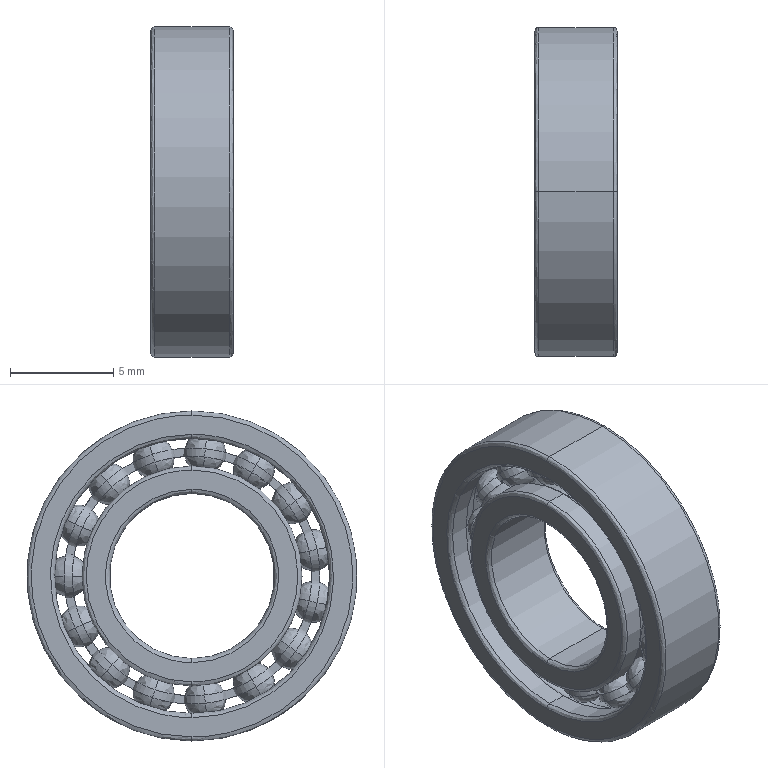Part | SolidWorks | features BaseBody 17 | 17 solids | 189 faces | box 4 x 16 x 16 mm | volume 445.743 mm3 | spline 85 | cylinder 70 | plane 34 | commonest cylinder face diameters 11.6 x29 12.4 x29 10.667 x4 13.333 x4 8 x2 16 x2